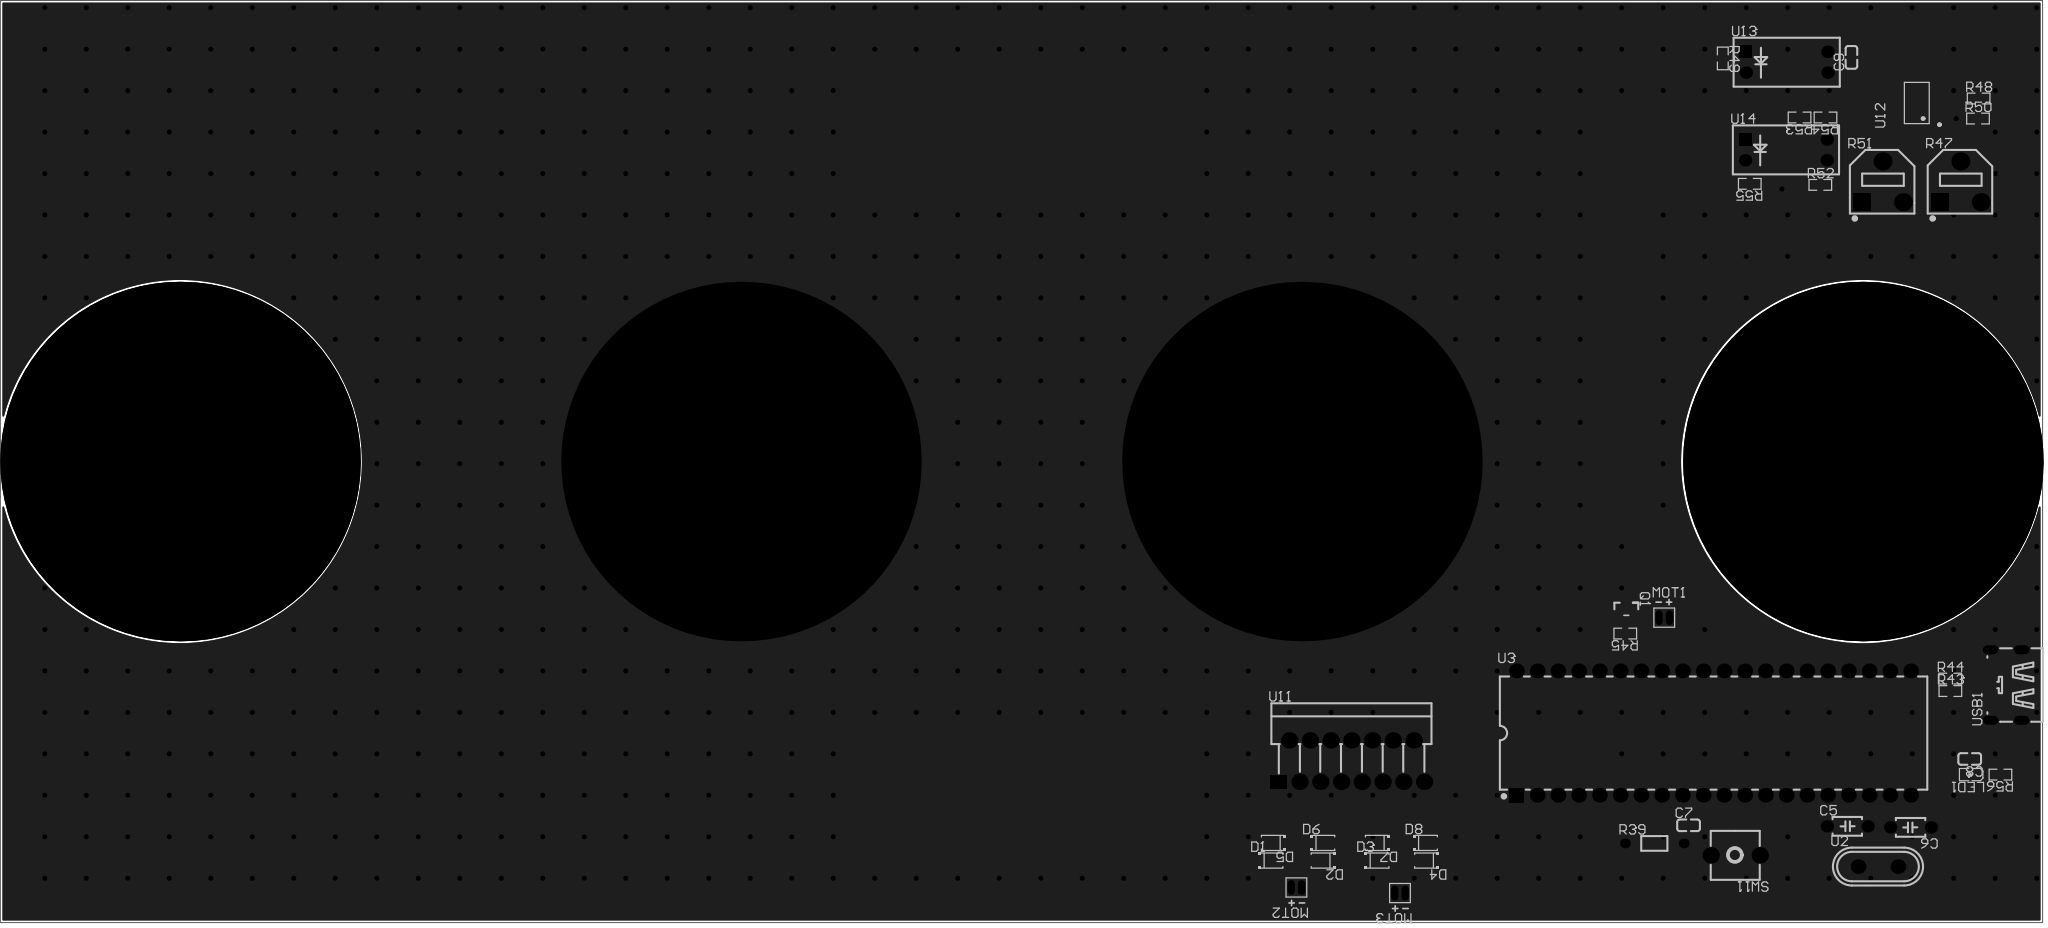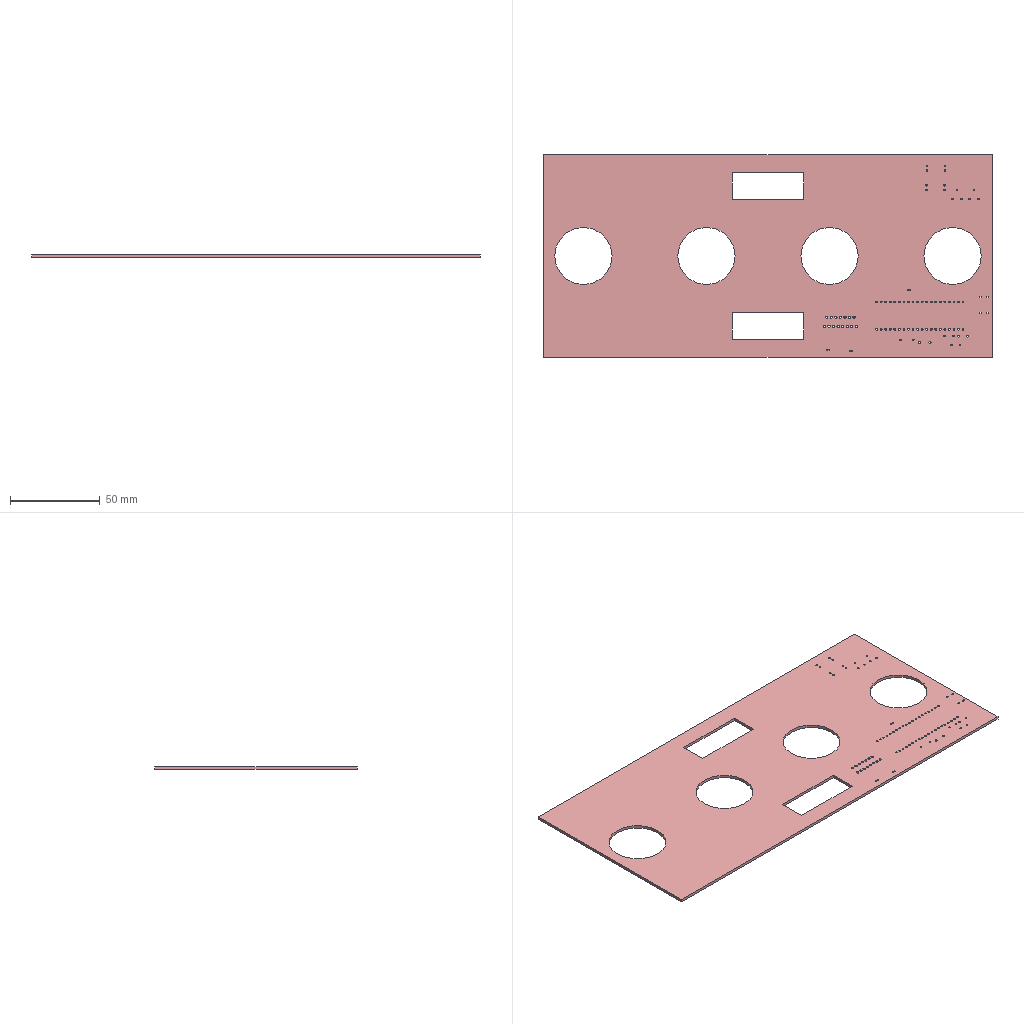Circuit board layout | Altium Designer | box 250 x 113 x 1.6 mm
Layer stack:
# Altium Designer layer stack of  (unit mm; dielectric type: 0 none, 1 core, 2 prepreg, 3 surface material)
index,name,kind,layer,copper_thickness_mm,dielectric_type,dielectric_thickness_mm,dielectric_material,dielectric_constant
0,Top Paste Mask Layer,other,,,,,,
1,Top Silkscreen Layer,other,,,,,,
2,Top Solder Mask Layer,dielectric,,,3,0.01,,3.3
3,Top Layer,copper,Top Layer,0.035,,,,
4,SUBSTRATE1,dielectric,,,3,1.51,FR4,4.5
5,Bottom Layer,copper,Bottom Layer,0.035,,,,
6,Bottom Solder Mask Layer,dielectric,,,3,0.01,,3.3
7,Bottom Silkscreen Layer,other,,,,,,
8,Bottom Paste Mask Layer,other,,,,,,
# drill layer pairs: low layer,high layer
drill_pair,Top Layer,Bottom Layer
Part placement:
Designator,Comment,Layer,Footprint,Center-X(mm),Center-Y(mm),Rotation
C5,22pF,TopLayer,CAP-TH_L3.6-W2.3-P5.00-D0.5,311.277,109.22,0
C6,22pF,TopLayer,CAP-TH_L3.6-W2.3-P5.00-D0.5,319.024,109.093,180
C7,100pF,TopLayer,C0603,291.846,109.347,0
C8,100nF,TopLayer,C0603,326.263,117.475,180
C9,100nF,TopLayer,C0603,311.785,203.454,90
D1,,TopLayer,SOD-123FL_L2.7-W1.8-LS3.8-RD,240.807,105.025,0
D2,,TopLayer,SOD-123FL_L2.7-W1.8-LS3.8-RD,247.03,105.025,180
D3,,TopLayer,SOD-123FL_L2.7-W1.8-LS3.8-RD,253.789,105.025,0
D4,,TopLayer,SOD-123FL_L2.7-W1.8-LS3.8-RD,259.695,105.025,180
D5,,TopLayer,SOD-123FL_L2.7-W1.8-LS3.8-RD,240.934,107.184,180
D6,,TopLayer,SOD-123FL_L2.7-W1.8-LS3.8-RD,247.157,107.184,0
D7,,TopLayer,SOD-123FL_L2.7-W1.8-LS3.8-RD,253.662,107.184,180
D8,,TopLayer,SOD-123FL_L2.7-W1.8-LS3.8-RD,259.715,107.188,0
LED1,,TopLayer,LED_0603,326.393,115.565,180
MOT1,LCM1027A2445F,TopLayer,VIBRATING-MOTOR-SMD_WELDING,288.87,134.797,0
MOT2,LCM1027A2445F,TopLayer,VIBRATING-MOTOR-SMD_WELDING,243.84,101.727,180
MOT3,LCM1027A2445F,TopLayer,VIBRATING-MOTOR-SMD_WELDING,256.52,101.044,180
Q1,,TopLayer,S8550P_SOT,284.226,135.975,270
R39,10kΩ,TopLayer,Res_1/8W,287.655,107.124,0
R43,5.1K,TopLayer,R0603,323.894,125.799,0
R44,5.1K,TopLayer,R0603,323.886,127.325,0
R45,1K,TopLayer,R0603,284.099,132.842,180
R47,10kΩ,TopLayer,RES-ADJ-SMD_RM065-V1,325.12,188.214,0
R48,10K,TopLayer,R0603,327.355,198.414,0
R49,100K,TopLayer,R0603,296.037,203.327,270
R50,10K,TopLayer,R0603,327.279,195.961,0
R51,10kΩ,TopLayer,RES-ADJ-SMD_RM065-V1,315.595,188.214,0
R52,47K,TopLayer,R0603,307.975,187.833,0
R53,10K,TopLayer,R0603,305.435,196.088,180
R54,1K,TopLayer,R0603,308.61,196.088,180
R55,10K,TopLayer,R0603,299.339,187.96,180
SW11,Tactile switch, 6*6*5 plastic head, 260G, travel 0.25mm, through-hole 2-pin,TopLayer,KEY-TH_2P-L6.0-W6.0-P5.00,297.561,105.664,180
U2,12MHz,TopLayer,HC-49US_L11.0-W4.6-P4.88,315.036,104.289,0
U3,AT89C51,TopLayer,DIP-40_L52.3-W13.9-P2.54-LS15.2-BL,294.91,120.648,0
U11,L298N,TopLayer,MULTIWATT-15_L19.6-W5.0-P1.27-L,250.578,117.209,0
U12,LM393M,TopLayer,SOIC-8_L4.9-W3.9-P1.27-LS6.0-BL,319.786,197.866,90
U13,XL-ITR9707,TopLayer,OPTO-TH_4P-P2.54-XL-ITR9608,303.86,202.863,0
U14,XL-ITR9707,TopLayer,OPTO-TH_4P-P2.54-XL-ITR9608,303.769,192.119,0
USB1,TYPE_C_SMD_6P,TopLayer,TYPE-C-SMD_TYPE-C-6P,330.598,126.539,90
R56,1K,TopLayer,R0603,330.025,115.557,180
Pad and via stacks:
# Altium Designer via and pad stacks of  (unit mm). Each distinct definition once, with the count of objects using it.
# via: kind,start_layer,end_layer,hole_mm,diameter_mm,mode(0 simple;1 top-mid-bottom;2 full stack),diameter_per_layer,count,example_net
# pad: kind,layer,hole_mm,hole_type(0 round;1 square;2 slot),plating,top_size,top_shape(1 round;2 rect;3 octagon;9 rounded rect),mid_size,bottom_size,mode,footprint,size_per_layer,count,example
pad,Multi-Layer,32,0,plated,44x44,1,44x44,44x44,0,,,4,1
pad,Multi-Layer,0.9,0,plated,1.5x1.5,1,1.5x1.5,1.5x1.5,0,CAP-TH_L3.6-W2.3-P5.00-D0.5,,4,C5.1
pad,Multi-Layer,0.6096,0,plated,0.9x1.8,1,0.9x1.8,0.9x1.8,0,VIBRATING-MOTOR-SMD_WELDING,,6,MOT1.1
pad,Multi-Layer,0.8001,0,plated,1.199x1.199,1,1.199x1.199,1.199x1.199,0,Res_1/8W,,2,R39.1
pad,Multi-Layer,1,0,plated,2.2x2.1,2,2.2x2.1,2.2x2.1,0,RES-ADJ-SMD_RM065-V1,,2,R47.1
pad,Multi-Layer,1,0,plated,2.2x2.2,1,2.2x2.2,2.2x2.2,0,RES-ADJ-SMD_RM065-V1,,4,R47.3
pad,Multi-Layer,1.2,0,plated,2x2,1,2x2,2x2,0,KEY-TH_2P-L6.0-W6.0-P5.00,,2,SW11.2
pad,Multi-Layer,0.8,0,plated,1.8x1.8,1,1.8x1.8,1.8x1.8,0,HC-49US_L11.0-W4.6-P4.88,,2,U2.1
pad,Multi-Layer,1,0,plated,1.8x1.8,1,1.8x1.8,1.8x1.8,0,DIP-40_L52.3-W13.9-P2.54-LS15.2-BL,,39,U3.19
pad,Multi-Layer,1,0,plated,1.8x1.8,2,1.8x1.8,1.8x1.8,0,DIP-40_L52.3-W13.9-P2.54-LS15.2-BL,,1,U3.1
pad,Multi-Layer,1.3,0,plated,2x2,1,2x2,2x2,0,MULTIWATT-15_L19.6-W5.0-P1.27-L,,14,U11.15
pad,Multi-Layer,1.3,0,plated,2x1.6,2,2x1.6,2x1.6,0,MULTIWATT-15_L19.6-W5.0-P1.27-L,,1,U11.1
pad,Multi-Layer,0.9144,0,plated,1.524x1.524,1,1.524x1.524,1.524x1.524,0,OPTO-TH_4P-P2.54-XL-ITR9608,,6,U13.4
pad,Multi-Layer,0.9144,0,plated,1.524x1.524,2,1.524x1.524,1.524x1.524,0,OPTO-TH_4P-P2.54-XL-ITR9608,,2,U13.1
pad,Multi-Layer,0.7,2,plated,1.1x1.9,1,1.1x1.9,1.1x1.9,0,TYPE-C-SMD_TYPE-C-6P,,4,USB1.7
pad,Top Layer,0,0,plated,0.8x0.9,2,0.8x0.9,0.8x0.9,0,C0603,,6,C7.2
pad,Top Layer,0,0,plated,1.399x1.199,2,1.399x1.199,1.399x1.199,0,SOD-123FL_L2.7-W1.8-LS3.8-RD,,16,D1.2
pad,Top Layer,0,0,plated,0.8001x0.8001,2,0.8001x0.8001,0.8001x0.8001,0,LED_0603,,2,LED1.1
pad,Top Layer,0,0,plated,0.701x1.25,2,0.701x1.25,0.701x1.25,0,S8550P_SOT,,3,Q1.3
pad,Top Layer,0,0,plated,0.8065x0.864,2,0.8065x0.864,0.8065x0.864,0,R0603,,22,R43.2
pad,Top Layer,0,0,plated,0.588x2.045,1,0.588x2.045,0.588x2.045,0,SOIC-8_L4.9-W3.9-P1.27-LS6.0-BL,,8,U12.1
pad,Top Layer,0,0,plated,0.8x1.2,2,0.8x1.2,0.8x1.2,0,TYPE-C-SMD_TYPE-C-6P,,2,USB1.B12
pad,Top Layer,0,0,plated,0.7x1.2,2,0.7x1.2,0.7x1.2,0,TYPE-C-SMD_TYPE-C-6P,,4,USB1.B9
via,Top Layer,Bottom Layer,0.3048,0.61,0,,697,FANGDIELUO
Copper pours:
name,layer,net,type(0 solid;1 hatched;2 none)
Top Layer-GND,Top Layer,GND,0
Bottom Layer-GND,Bottom Layer,GND,0